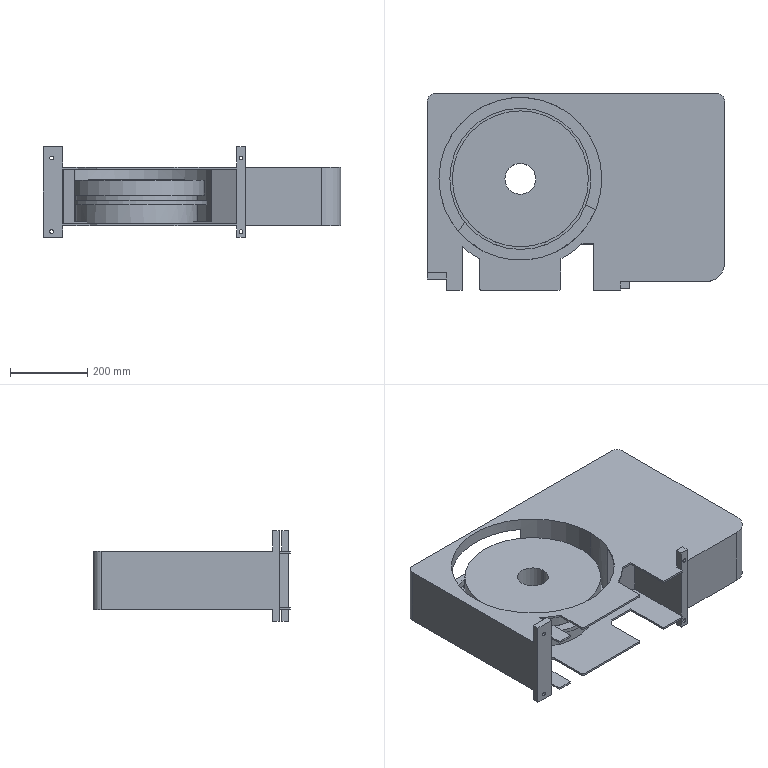Part | SolidWorks | features ICE 11, Fillet 2, Cut 1, Revolution 1 | 1 solid | 119 faces | box 770 x 509 x 235 mm | volume 22102054 mm3 | plane 76 | cylinder 43 | commonest cylinder face diameters 10 x12 20 x5 315.35 x5 40 x2 80 x2 104 x2